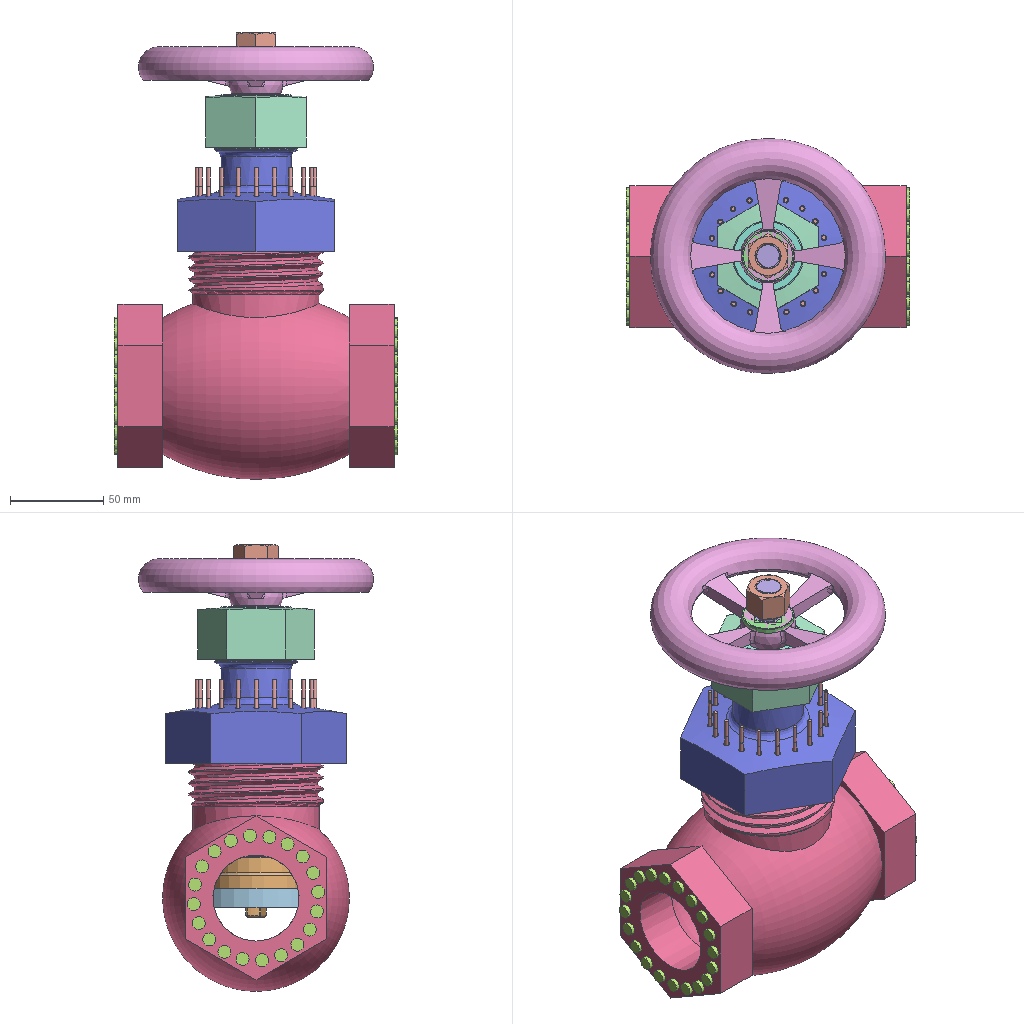Assembly | NX | 15 different items | 112 placed | box 152 x 126 x 239 mm
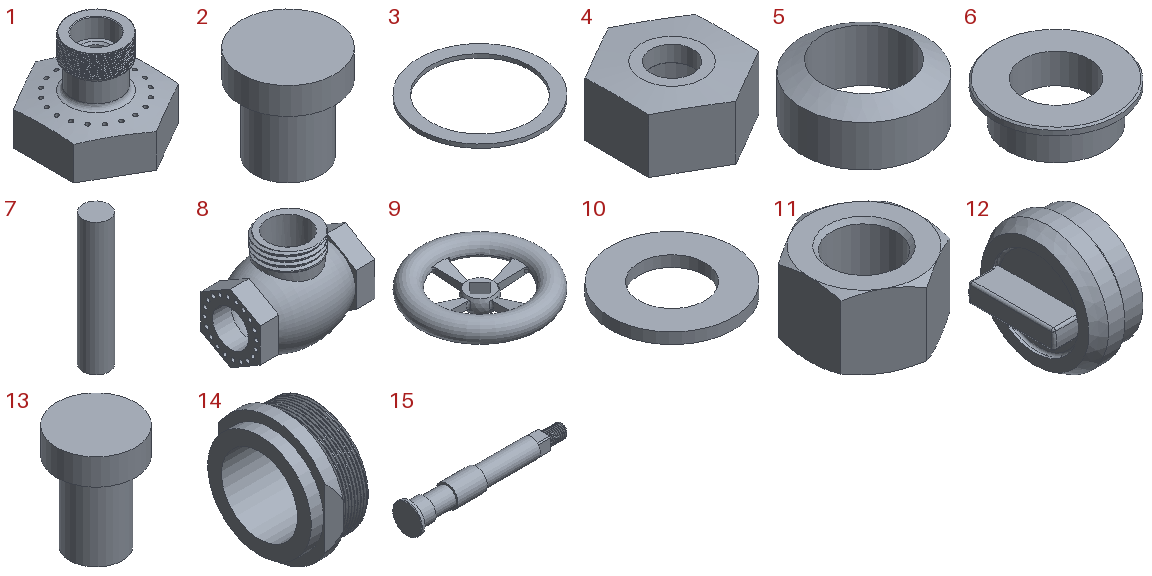Parts list (item | quantity | size | volume | features):
1 | x1 | 84 x 96.995 x 72 mm | 147613 mm3 | features CYLINDER 5, DATUM_CSYS 5, SKETCH 4, BLEND 3, CHAMFER 2, EXTRUDE 2, HOLE PACKAGE 2, SIMPLE HOLE 2, SWP104 2, THREADS 2, REPLACE_FACE 1, SYMBOLIC_THREAD 1
2 | x40 | 7 x 7 x 7 mm | 175.144 mm3 | features CYLINDER 2, DATUM_CSYS 1
3 | x1 | 65 x 65 x 2 mm | 2389 mm3 | features CYLINDER 2, DATUM_CSYS 1
4 | x1 | 54.002 x 62.354 x 28 mm | 36749 mm3 | features DATUM_CSYS 3, CYLINDER 2, SKETCH 2, CHAMFER 1, EXTRUDE 1, HOLE PACKAGE 1, SIMPLE HOLE 1, SWP104 1, SYMBOLIC_THREAD 1
5 | x1 | 30 x 30 x 12.74 mm | 4252 mm3 | features CYLINDER 2, CHAMFER 1, DATUM_CSYS 1
6 | x1 | 38 x 38 x 12 mm | 4882 mm3 | features DATUM_CSYS 2, BLEND 1, CHAMFER 1, SKETCH 1, SWP104 1
7 | x40 | 2 x 2 x 10 mm | 31.416 mm3 | features CYLINDER 1, DATUM_CSYS 1
8 | x1 | 148 x 100 x 122 mm | 413205 mm3 | features DATUM_CSYS 9, SKETCH 8, CYLINDER 7, EXTRUDE 6, EXTRACT_FACE 4, SYMBOLIC_THREAD 3, EXTRACT_DATUM_AXIS 2, Instance Feature 2, Mirror Feature 2, BLEND 1, CHAMFER 1, DATUM_PLANE 1, HOLE PACKAGE 1, REPLACE_FACE 1, SIMPLE HOLE 1, SWP104 1, THREADS 1
9 | x1 | 126 x 126 x 25 mm | 72074 mm3 | features DATUM_CSYS 12, SKETCH 11, EXTRUDE 10, EXTRACT_DATUM_AXIS 8, EXTRACT_DATUM_PLANE 8, EXTRACT_FACE 8, EXTRACT_STRING 8, Instance Feature 6, BLEND 5, INTERSECT 4, Pattern Feature 2, UNITE 2, SPHERE 1, SWP104 1
10 | x1 | 28 x 28 x 2.5 mm | 1098 mm3 | features CYLINDER 2, DATUM_CSYS 1
11 | x1 | 21 x 24.249 x 14.1 mm | 3611 mm3 | features DATUM_CSYS 4, EXTRUDE 3, SKETCH 3, EXTRACT_FACE 2, EXTRACT_STRING 2, HOLE PACKAGE 1, Instance Feature 1, Mirror Feature 1, SIMPLE HOLE 1, SYMBOLIC_THREAD 1
12 | x1 | 32 x 51 x 51 mm | 28582 mm3 | features BLEND 3, DATUM_CSYS 3, SKETCH 2, CHAMFER 1, CYLINDER 1, EXTRUDE 1, HOLE PACKAGE 1, SIMPLE HOLE 1, SWP104 1, SYMBOLIC_THREAD 1
13 | x20 | 3 x 3 x 4 mm | 16.493 mm3 | features CYLINDER 2, DATUM_CSYS 1
14 | x1 | 18 x 39.042 x 40 mm | 9368 mm3 | features DATUM_CSYS 3, SKETCH 2, THREADS 2, EXTRUDE 1, SWP104 1
15 | x1 | 168 x 32 x 32 mm | 56183 mm3 | features DATUM_CSYS 3, SKETCH 2, CHAMFER 1, EXTRUDE 1, SWP104 1, THREADS 1
Mates (type | each side: item.copy, entity, surface, feature):
Concentric | 12.1 edge | 8.1 edge
Concentric | 14.1 edge | 12.1 edge
Concentric | 15.1 edge | 14.1 edge
Concentric | 1.1 edge | 8.1 edge
Concentric | 1.1 edge | 5.1 edge
Concentric | 6.1 edge | 4.1 edge
Concentric | 9.1 edge | 15.1 edge
Concentric | 11.1 edge | 15.1 edge
Concentric | 10.1 edge | 9.1 edge
Concentric | 3.1 edge | 14.1 edge
Concentric | 2.1 edge | 8.1 edge | 2 times
Concentric | 13.1 edge | 1.1 edge
Concentric | 7.1 edge | 13.1 edge
Concentric | 7.1 edge | 7.1 edge